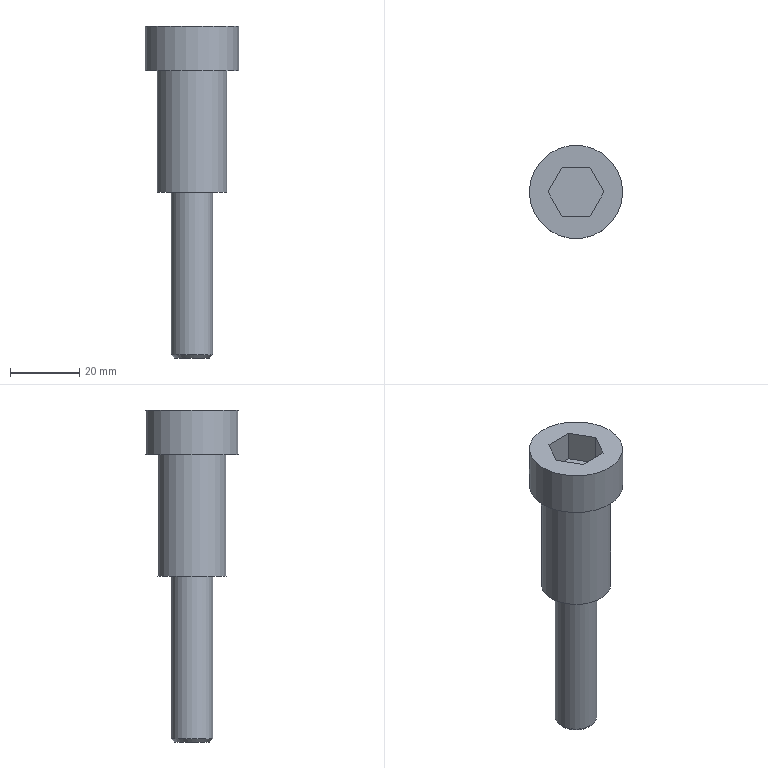Part | STEP file | 1_id554_xmt_txt | 1 solid | 15 faces | box 27 x 27 x 96 mm | volume 22322 mm3 | plane 11 | cylinder 3 | cone 1 | commonest cylinder face diameters 12 x1 20 x1 27 x1
STEP:
#1=CARTESIAN_POINT('',(151.5,-55.,184.));
#2=VERTEX_POINT('',#1);
#3=CARTESIAN_POINT('',(165.,-55.,184.));
#4=DIRECTION('',(0.,0.,1.));
#5=DIRECTION('',(-1.,0.,0.));
#6=AXIS2_PLACEMENT_3D('',#3,#4,#5);
#7=CIRCLE('',#6,13.5);
#8=EDGE_CURVE('',#2,#2,#7,.T.);
#9=ORIENTED_EDGE('',*,*,#8,.F.);
#10=EDGE_LOOP('',(#9));
#11=FACE_BOUND('',#10,.T.);
#12=CARTESIAN_POINT('',(151.5,-55.,171.));
#13=VERTEX_POINT('',#12);
#14=CARTESIAN_POINT('',(165.,-55.,171.));
#15=DIRECTION('',(0.,0.,-1.));
#16=DIRECTION('',(-1.,0.,0.));
#17=AXIS2_PLACEMENT_3D('',#14,#15,#16);
#18=CIRCLE('',#17,13.5);
#19=EDGE_CURVE('',#13,#13,#18,.T.);
#20=ORIENTED_EDGE('',*,*,#19,.F.);
#21=EDGE_LOOP('',(#20));
#22=FACE_BOUND('',#21,.T.);
#23=CARTESIAN_POINT('',(165.,-55.,177.5));
#24=DIRECTION('',(0.,0.,-1.));
#25=DIRECTION('',(1.,0.,0.));
#26=AXIS2_PLACEMENT_3D('',#23,#24,#25);
#27=CYLINDRICAL_SURFACE('',#26,13.5);
#28=ADVANCED_FACE('',(#11,#22),#27,.T.);
#29=CARTESIAN_POINT('',(155.,-55.,171.));
#30=VERTEX_POINT('',#29);
#31=CARTESIAN_POINT('',(165.,-55.,171.));
#32=DIRECTION('',(0.,0.,1.));
#33=DIRECTION('',(-1.,0.,0.));
#34=AXIS2_PLACEMENT_3D('',#31,#32,#33);
#35=CIRCLE('',#34,10.);
#36=EDGE_CURVE('',#30,#30,#35,.T.);
#37=ORIENTED_EDGE('',*,*,#36,.F.);
#38=EDGE_LOOP('',(#37));
#39=FACE_BOUND('',#38,.T.);
#40=CARTESIAN_POINT('',(155.,-55.,136.));
#41=VERTEX_POINT('',#40);
#42=CARTESIAN_POINT('',(165.,-55.,136.));
#43=DIRECTION('',(0.,0.,-1.));
#44=DIRECTION('',(-1.,0.,0.));
#45=AXIS2_PLACEMENT_3D('',#42,#43,#44);
#46=CIRCLE('',#45,10.);
#47=EDGE_CURVE('',#41,#41,#46,.T.);
#48=ORIENTED_EDGE('',*,*,#47,.F.);
#49=EDGE_LOOP('',(#48));
#50=FACE_BOUND('',#49,.T.);
#51=CARTESIAN_POINT('',(165.,-55.,153.5));
#52=DIRECTION('',(0.,0.,-1.));
#53=DIRECTION('',(1.,0.,0.));
#54=AXIS2_PLACEMENT_3D('',#51,#52,#53);
#55=CYLINDRICAL_SURFACE('',#54,10.);
#56=ADVANCED_FACE('',(#39,#50),#55,.T.);
#57=CARTESIAN_POINT('',(159.,-55.,89.));
#58=VERTEX_POINT('',#57);
#59=CARTESIAN_POINT('',(165.,-55.,89.));
#60=DIRECTION('',(0.,0.,1.));
#61=DIRECTION('',(-1.,0.,0.));
#62=AXIS2_PLACEMENT_3D('',#59,#60,#61);
#63=CIRCLE('',#62,6.);
#64=EDGE_CURVE('',#58,#58,#63,.T.);
#65=ORIENTED_EDGE('',*,*,#64,.T.);
#66=EDGE_LOOP('',(#65));
#67=FACE_BOUND('',#66,.T.);
#68=CARTESIAN_POINT('',(159.,-55.,136.));
#69=VERTEX_POINT('',#68);
#70=CARTESIAN_POINT('',(165.,-55.,136.));
#71=DIRECTION('',(0.,0.,1.));
#72=DIRECTION('',(-1.,0.,0.));
#73=AXIS2_PLACEMENT_3D('',#70,#71,#72);
#74=CIRCLE('',#73,6.);
#75=EDGE_CURVE('',#69,#69,#74,.T.);
#76=ORIENTED_EDGE('',*,*,#75,.F.);
#77=EDGE_LOOP('',(#76));
#78=FACE_BOUND('',#77,.T.);
#79=CARTESIAN_POINT('',(165.,-55.,112.));
#80=DIRECTION('',(0.,0.,-1.));
#81=DIRECTION('',(1.,0.,0.));
#82=AXIS2_PLACEMENT_3D('',#79,#80,#81);
#83=CYLINDRICAL_SURFACE('',#82,6.);
#84=ADVANCED_FACE('',(#67,#78),#83,.T.);
#85=CARTESIAN_POINT('',(169.041,-48.,175.));
#86=VERTEX_POINT('',#85);
#87=CARTESIAN_POINT('',(160.959,-48.,175.));
#88=VERTEX_POINT('',#87);
#89=CARTESIAN_POINT('',(169.041,-48.,175.));
#90=DIRECTION('',(-1.,0.,0.));
#91=VECTOR('',#90,1.);
#92=LINE('',#89,#91);
#93=EDGE_CURVE('',#86,#88,#92,.T.);
#94=ORIENTED_EDGE('',*,*,#93,.F.);
#95=CARTESIAN_POINT('',(169.041,-48.,184.));
#96=VERTEX_POINT('',#95);
#97=CARTESIAN_POINT('',(169.041,-48.,184.));
#98=DIRECTION('',(0.,0.,-1.));
#99=VECTOR('',#98,1.);
#100=LINE('',#97,#99);
#101=EDGE_CURVE('',#96,#86,#100,.T.);
#102=ORIENTED_EDGE('',*,*,#101,.F.);
#103=CARTESIAN_POINT('',(160.959,-48.,184.));
#104=VERTEX_POINT('',#103);
#105=CARTESIAN_POINT('',(165.,-48.,184.));
#106=DIRECTION('',(1.,0.,0.));
#107=VECTOR('',#106,1.);
#108=LINE('',#105,#107);
#109=EDGE_CURVE('',#104,#96,#108,.T.);
#110=ORIENTED_EDGE('',*,*,#109,.F.);
#111=CARTESIAN_POINT('',(160.959,-48.,184.));
#112=DIRECTION('',(0.,0.,-1.));
#113=VECTOR('',#112,1.);
#114=LINE('',#111,#113);
#115=EDGE_CURVE('',#104,#88,#114,.T.);
#116=ORIENTED_EDGE('',*,*,#115,.T.);
#117=EDGE_LOOP('',(#94,#102,#110,#116));
#118=FACE_OUTER_BOUND('',#117,.T.);
#119=CARTESIAN_POINT('',(165.,-48.,184.));
#120=DIRECTION('',(0.,1.,0.));
#121=DIRECTION('',(-1.,0.,0.));
#122=AXIS2_PLACEMENT_3D('',#119,#120,#121);
#123=PLANE('',#122);
#124=ADVANCED_FACE('',(#118),#123,.F.);
#125=CARTESIAN_POINT('',(156.917,-55.,175.));
#126=VERTEX_POINT('',#125);
#127=CARTESIAN_POINT('',(160.959,-48.,175.));
#128=DIRECTION('',(-0.5,-0.866,0.));
#129=VECTOR('',#128,1.);
#130=LINE('',#127,#129);
#131=EDGE_CURVE('',#88,#126,#130,.T.);
#132=ORIENTED_EDGE('',*,*,#131,.F.);
#133=ORIENTED_EDGE('',*,*,#115,.F.);
#134=CARTESIAN_POINT('',(156.917,-55.,184.));
#135=VERTEX_POINT('',#134);
#136=CARTESIAN_POINT('',(158.938,-51.5,184.));
#137=DIRECTION('',(0.5,0.866,0.));
#138=VECTOR('',#137,1.);
#139=LINE('',#136,#138);
#140=EDGE_CURVE('',#135,#104,#139,.T.);
#141=ORIENTED_EDGE('',*,*,#140,.F.);
#142=CARTESIAN_POINT('',(156.917,-55.,184.));
#143=DIRECTION('',(0.,0.,-1.));
#144=VECTOR('',#143,1.);
#145=LINE('',#142,#144);
#146=EDGE_CURVE('',#135,#126,#145,.T.);
#147=ORIENTED_EDGE('',*,*,#146,.T.);
#148=EDGE_LOOP('',(#132,#133,#141,#147));
#149=FACE_OUTER_BOUND('',#148,.T.);
#150=CARTESIAN_POINT('',(158.938,-51.5,184.));
#151=DIRECTION('',(-0.866,0.5,0.));
#152=DIRECTION('',(-0.5,-0.866,0.));
#153=AXIS2_PLACEMENT_3D('',#150,#151,#152);
#154=PLANE('',#153);
#155=ADVANCED_FACE('',(#149),#154,.F.);
#156=CARTESIAN_POINT('',(160.959,-62.,175.));
#157=VERTEX_POINT('',#156);
#158=CARTESIAN_POINT('',(156.917,-55.,175.));
#159=DIRECTION('',(0.5,-0.866,0.));
#160=VECTOR('',#159,1.);
#161=LINE('',#158,#160);
#162=EDGE_CURVE('',#126,#157,#161,.T.);
#163=ORIENTED_EDGE('',*,*,#162,.F.);
#164=ORIENTED_EDGE('',*,*,#146,.F.);
#165=CARTESIAN_POINT('',(160.959,-62.,184.));
#166=VERTEX_POINT('',#165);
#167=CARTESIAN_POINT('',(158.938,-58.5,184.));
#168=DIRECTION('',(-0.5,0.866,0.));
#169=VECTOR('',#168,1.);
#170=LINE('',#167,#169);
#171=EDGE_CURVE('',#166,#135,#170,.T.);
#172=ORIENTED_EDGE('',*,*,#171,.F.);
#173=CARTESIAN_POINT('',(160.959,-62.,184.));
#174=DIRECTION('',(0.,0.,-1.));
#175=VECTOR('',#174,1.);
#176=LINE('',#173,#175);
#177=EDGE_CURVE('',#166,#157,#176,.T.);
#178=ORIENTED_EDGE('',*,*,#177,.T.);
#179=EDGE_LOOP('',(#163,#164,#172,#178));
#180=FACE_OUTER_BOUND('',#179,.T.);
#181=CARTESIAN_POINT('',(158.938,-58.5,184.));
#182=DIRECTION('',(-0.866,-0.5,0.));
#183=DIRECTION('',(0.5,-0.866,0.));
#184=AXIS2_PLACEMENT_3D('',#181,#182,#183);
#185=PLANE('',#184);
#186=ADVANCED_FACE('',(#180),#185,.F.);
#187=CARTESIAN_POINT('',(169.041,-62.,175.));
#188=VERTEX_POINT('',#187);
#189=CARTESIAN_POINT('',(160.959,-62.,175.));
#190=DIRECTION('',(1.,0.,0.));
#191=VECTOR('',#190,1.);
#192=LINE('',#189,#191);
#193=EDGE_CURVE('',#157,#188,#192,.T.);
#194=ORIENTED_EDGE('',*,*,#193,.F.);
#195=ORIENTED_EDGE('',*,*,#177,.F.);
#196=CARTESIAN_POINT('',(169.041,-62.,184.));
#197=VERTEX_POINT('',#196);
#198=CARTESIAN_POINT('',(165.,-62.,184.));
#199=DIRECTION('',(-1.,0.,0.));
#200=VECTOR('',#199,1.);
#201=LINE('',#198,#200);
#202=EDGE_CURVE('',#197,#166,#201,.T.);
#203=ORIENTED_EDGE('',*,*,#202,.F.);
#204=CARTESIAN_POINT('',(169.041,-62.,184.));
#205=DIRECTION('',(0.,0.,-1.));
#206=VECTOR('',#205,1.);
#207=LINE('',#204,#206);
#208=EDGE_CURVE('',#197,#188,#207,.T.);
#209=ORIENTED_EDGE('',*,*,#208,.T.);
#210=EDGE_LOOP('',(#194,#195,#203,#209));
#211=FACE_OUTER_BOUND('',#210,.T.);
#212=CARTESIAN_POINT('',(165.,-62.,184.));
#213=DIRECTION('',(0.,-1.,0.));
#214=DIRECTION('',(1.,0.,0.));
#215=AXIS2_PLACEMENT_3D('',#212,#213,#214);
#216=PLANE('',#215);
#217=ADVANCED_FACE('',(#211),#216,.F.);
#218=CARTESIAN_POINT('',(173.083,-55.,175.));
#219=VERTEX_POINT('',#218);
#220=CARTESIAN_POINT('',(169.041,-62.,175.));
#221=DIRECTION('',(0.5,0.866,0.));
#222=VECTOR('',#221,1.);
#223=LINE('',#220,#222);
#224=EDGE_CURVE('',#188,#219,#223,.T.);
#225=ORIENTED_EDGE('',*,*,#224,.F.);
#226=ORIENTED_EDGE('',*,*,#208,.F.);
#227=CARTESIAN_POINT('',(173.083,-55.,184.));
#228=VERTEX_POINT('',#227);
#229=CARTESIAN_POINT('',(171.062,-58.5,184.));
#230=DIRECTION('',(-0.5,-0.866,0.));
#231=VECTOR('',#230,1.);
#232=LINE('',#229,#231);
#233=EDGE_CURVE('',#228,#197,#232,.T.);
#234=ORIENTED_EDGE('',*,*,#233,.F.);
#235=CARTESIAN_POINT('',(173.083,-55.,184.));
#236=DIRECTION('',(0.,0.,-1.));
#237=VECTOR('',#236,1.);
#238=LINE('',#235,#237);
#239=EDGE_CURVE('',#228,#219,#238,.T.);
#240=ORIENTED_EDGE('',*,*,#239,.T.);
#241=EDGE_LOOP('',(#225,#226,#234,#240));
#242=FACE_OUTER_BOUND('',#241,.T.);
#243=CARTESIAN_POINT('',(171.062,-58.5,184.));
#244=DIRECTION('',(0.866,-0.5,0.));
#245=DIRECTION('',(0.5,0.866,0.));
#246=AXIS2_PLACEMENT_3D('',#243,#244,#245);
#247=PLANE('',#246);
#248=ADVANCED_FACE('',(#242),#247,.F.);
#249=CARTESIAN_POINT('',(173.083,-55.,175.));
#250=DIRECTION('',(-0.5,0.866,0.));
#251=VECTOR('',#250,1.);
#252=LINE('',#249,#251);
#253=EDGE_CURVE('',#219,#86,#252,.T.);
#254=ORIENTED_EDGE('',*,*,#253,.F.);
#255=ORIENTED_EDGE('',*,*,#239,.F.);
#256=CARTESIAN_POINT('',(171.062,-51.5,184.));
#257=DIRECTION('',(0.5,-0.866,0.));
#258=VECTOR('',#257,1.);
#259=LINE('',#256,#258);
#260=EDGE_CURVE('',#96,#228,#259,.T.);
#261=ORIENTED_EDGE('',*,*,#260,.F.);
#262=ORIENTED_EDGE('',*,*,#101,.T.);
#263=EDGE_LOOP('',(#254,#255,#261,#262));
#264=FACE_OUTER_BOUND('',#263,.T.);
#265=CARTESIAN_POINT('',(171.062,-51.5,184.));
#266=DIRECTION('',(0.866,0.5,0.));
#267=DIRECTION('',(-0.5,0.866,0.));
#268=AXIS2_PLACEMENT_3D('',#265,#266,#267);
#269=PLANE('',#268);
#270=ADVANCED_FACE('',(#264),#269,.F.);
#271=ORIENTED_EDGE('',*,*,#93,.T.);
#272=ORIENTED_EDGE('',*,*,#131,.T.);
#273=ORIENTED_EDGE('',*,*,#162,.T.);
#274=ORIENTED_EDGE('',*,*,#193,.T.);
#275=ORIENTED_EDGE('',*,*,#224,.T.);
#276=ORIENTED_EDGE('',*,*,#253,.T.);
#277=EDGE_LOOP('',(#271,#272,#273,#274,#275,#276));
#278=FACE_OUTER_BOUND('',#277,.T.);
#279=CARTESIAN_POINT('',(165.,-55.,175.));
#280=DIRECTION('',(0.,0.,-1.));
#281=DIRECTION('',(1.,0.,0.));
#282=AXIS2_PLACEMENT_3D('',#279,#280,#281);
#283=PLANE('',#282);
#284=ADVANCED_FACE('',(#278),#283,.F.);
#285=CARTESIAN_POINT('',(160.,-55.,88.));
#286=VERTEX_POINT('',#285);
#287=CARTESIAN_POINT('',(165.,-55.,88.));
#288=DIRECTION('',(0.,0.,-1.));
#289=DIRECTION('',(-1.,0.,0.));
#290=AXIS2_PLACEMENT_3D('',#287,#288,#289);
#291=CIRCLE('',#290,5.);
#292=EDGE_CURVE('',#286,#286,#291,.T.);
#293=ORIENTED_EDGE('',*,*,#292,.T.);
#294=EDGE_LOOP('',(#293));
#295=FACE_OUTER_BOUND('',#294,.T.);
#296=CARTESIAN_POINT('',(165.,-55.,88.));
#297=DIRECTION('',(0.,0.,-1.));
#298=DIRECTION('',(1.,0.,0.));
#299=AXIS2_PLACEMENT_3D('',#296,#297,#298);
#300=PLANE('',#299);
#301=ADVANCED_FACE('',(#295),#300,.T.);
#302=ORIENTED_EDGE('',*,*,#75,.T.);
#303=EDGE_LOOP('',(#302));
#304=FACE_BOUND('',#303,.T.);
#305=ORIENTED_EDGE('',*,*,#47,.T.);
#306=EDGE_LOOP('',(#305));
#307=FACE_BOUND('',#306,.T.);
#308=CARTESIAN_POINT('',(165.,-55.,136.));
#309=DIRECTION('',(0.,0.,-1.));
#310=DIRECTION('',(1.,0.,0.));
#311=AXIS2_PLACEMENT_3D('',#308,#309,#310);
#312=PLANE('',#311);
#313=ADVANCED_FACE('',(#304,#307),#312,.T.);
#314=ORIENTED_EDGE('',*,*,#109,.T.);
#315=ORIENTED_EDGE('',*,*,#260,.T.);
#316=ORIENTED_EDGE('',*,*,#233,.T.);
#317=ORIENTED_EDGE('',*,*,#202,.T.);
#318=ORIENTED_EDGE('',*,*,#171,.T.);
#319=ORIENTED_EDGE('',*,*,#140,.T.);
#320=EDGE_LOOP('',(#314,#315,#316,#317,#318,#319));
#321=FACE_BOUND('',#320,.T.);
#322=ORIENTED_EDGE('',*,*,#8,.T.);
#323=EDGE_LOOP('',(#322));
#324=FACE_BOUND('',#323,.T.);
#325=CARTESIAN_POINT('',(165.,-55.,184.));
#326=DIRECTION('',(0.,0.,1.));
#327=DIRECTION('',(-1.,0.,0.));
#328=AXIS2_PLACEMENT_3D('',#325,#326,#327);
#329=PLANE('',#328);
#330=ADVANCED_FACE('',(#321,#324),#329,.T.);
#331=ORIENTED_EDGE('',*,*,#36,.T.);
#332=EDGE_LOOP('',(#331));
#333=FACE_BOUND('',#332,.T.);
#334=ORIENTED_EDGE('',*,*,#19,.T.);
#335=EDGE_LOOP('',(#334));
#336=FACE_BOUND('',#335,.T.);
#337=CARTESIAN_POINT('',(165.,-55.,171.));
#338=DIRECTION('',(0.,0.,-1.));
#339=DIRECTION('',(1.,0.,0.));
#340=AXIS2_PLACEMENT_3D('',#337,#338,#339);
#341=PLANE('',#340);
#342=ADVANCED_FACE('',(#333,#336),#341,.T.);
#343=ORIENTED_EDGE('',*,*,#64,.F.);
#344=EDGE_LOOP('',(#343));
#345=FACE_BOUND('',#344,.T.);
#346=ORIENTED_EDGE('',*,*,#292,.F.);
#347=EDGE_LOOP('',(#346));
#348=FACE_BOUND('',#347,.T.);
#349=CARTESIAN_POINT('',(165.,-55.,88.));
#350=DIRECTION('',(0.,0.,1.));
#351=DIRECTION('',(1.,0.,0.));
#352=AXIS2_PLACEMENT_3D('',#349,#350,#351);
#353=CONICAL_SURFACE('',#352,5.,45.);
#354=ADVANCED_FACE('',(#345,#348),#353,.T.);
#355=CLOSED_SHELL('',(#28,#56,#84,#124,#155,#186,#217,#248,#270,#284,#301,#313,#330,#342,#354));
#356=MANIFOLD_SOLID_BREP('',#355);
#357=(LENGTH_UNIT()NAMED_UNIT(*)SI_UNIT(.MILLI.,.METRE.));
#358=UNCERTAINTY_MEASURE_WITH_UNIT(LENGTH_MEASURE(0.00002),#357,'','');
#359=(NAMED_UNIT(*)PLANE_ANGLE_UNIT()SI_UNIT($,.RADIAN.));
#360=PLANE_ANGLE_MEASURE_WITH_UNIT(PLANE_ANGLE_MEASURE(0.01745),#359);
#361=DIMENSIONAL_EXPONENTS(0.,0.,0.,0.,0.,0.,0.);
#362=(CONVERSION_BASED_UNIT('DEGREE',#360)NAMED_UNIT(#361)PLANE_ANGLE_UNIT());
#363=(NAMED_UNIT(*)SI_UNIT($,.STERADIAN.)SOLID_ANGLE_UNIT());
#364=(GEOMETRIC_REPRESENTATION_CONTEXT(3)GLOBAL_UNCERTAINTY_ASSIGNED_CONTEXT((#358))GLOBAL_UNIT_ASSIGNED_CONTEXT((#357,#362,#363))REPRESENTATION_CONTEXT('',''));
#365=ADVANCED_BREP_SHAPE_REPRESENTATION('',(#356),#364);